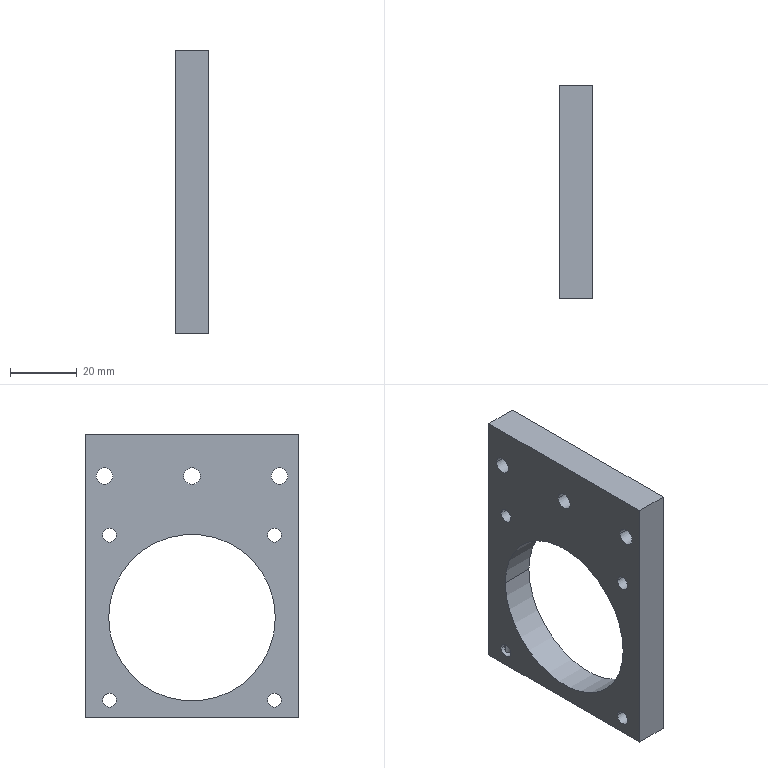Part | NX | 1 solid | 52 faces | box 10 x 64 x 85 mm | volume 33530 mm3 | cylinder 24 | cone 22 | plane 6 | commonest cylinder face diameters 2.5 x8 4.2 x8 5 x6 50 x2